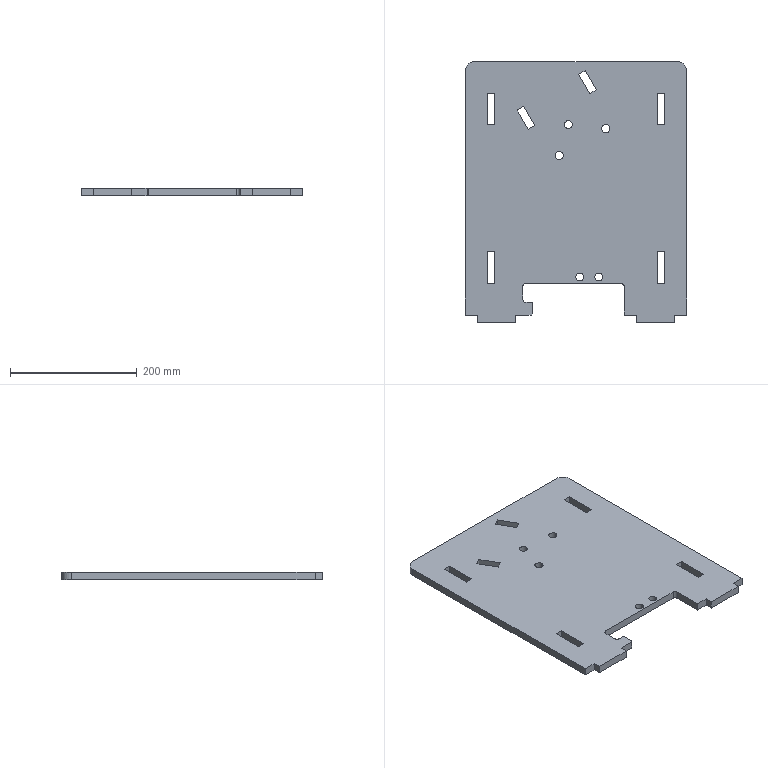Part | SolidWorks | features FlatPattern 1, SMBaseFlange 1, SheetMetal 1 | 1 solid | 60 faces | box 350 x 411.5 x 12 mm | volume 1556687 mm3 | plane 45 | cylinder 15 | commonest cylinder face diameters 12.5 x6 13 x4 10 x3 30 x2